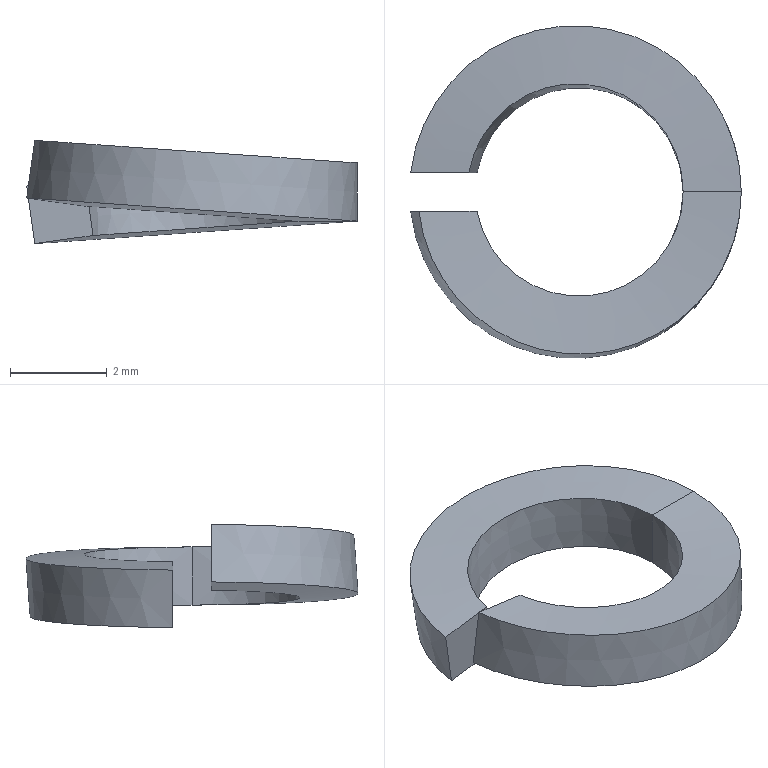Part | NX | features BREP 1 | 1 solid | 10 faces | box 6.827 x 6.867 x 2.131 mm | volume 24.116 mm3 | cone 8 | plane 2
STEP:
#1=CARTESIAN_POINT('',(-2.058,-0.4,1.498));
#2=VERTEX_POINT('',#1);
#3=CARTESIAN_POINT('',(-2.226,-0.4,0.3095));
#4=VERTEX_POINT('',#3);
#5=CARTESIAN_POINT('',(-2.058,-0.4,1.498));
#6=CARTESIAN_POINT('',(-2.084,-0.4,1.314));
#7=CARTESIAN_POINT('',(-2.11,-0.4,1.13));
#8=CARTESIAN_POINT('',(-2.161,-0.4,0.7669));
#9=CARTESIAN_POINT('',(-2.187,-0.4,0.5875));
#10=CARTESIAN_POINT('',(-2.217,-0.4,0.3753));
#11=CARTESIAN_POINT('',(-2.221,-0.4,0.3424));
#12=CARTESIAN_POINT('',(-2.226,-0.4,0.3095));
#13=B_SPLINE_CURVE_WITH_KNOTS('',3,(#5,#6,#7,#8,#9,#10,#11,#12),.UNSPECIFIED.,.F.,.F.,(4,2,2,4),(0.,0.4641,0.917,1.),.UNSPECIFIED.);
#14=EDGE_CURVE('',#2,#4,#13,.T.);
#15=ORIENTED_EDGE('',*,*,#14,.F.);
#16=CARTESIAN_POINT('',(2.2,0.,1.2));
#17=VERTEX_POINT('',#16);
#18=CARTESIAN_POINT('',(0.05246,0.,1.35));
#19=DIRECTION('',(0.06976,0.,0.9976));
#20=DIRECTION('',(0.9976,0.,-0.06976));
#21=AXIS2_PLACEMENT_3D('',#18,#19,#20);
#22=CIRCLE('',#21,2.153);
#23=EDGE_CURVE('',#2,#17,#22,.T.);
#24=ORIENTED_EDGE('',*,*,#23,.T.);
#25=CARTESIAN_POINT('',(2.2,0.,0.));
#26=VERTEX_POINT('',#25);
#27=CARTESIAN_POINT('',(2.2,0.,0.));
#28=DIRECTION('',(0.,0.,1.));
#29=VECTOR('',#28,1000.);
#30=LINE('',#27,#29);
#31=EDGE_CURVE('',#26,#17,#30,.T.);
#32=ORIENTED_EDGE('',*,*,#31,.F.);
#33=CARTESIAN_POINT('',(-0.03105,0.,0.156));
#34=DIRECTION('',(0.06976,0.,0.9976));
#35=DIRECTION('',(0.9976,0.,-0.06976));
#36=AXIS2_PLACEMENT_3D('',#33,#34,#35);
#37=CIRCLE('',#36,2.236);
#38=EDGE_CURVE('',#4,#26,#37,.T.);
#39=ORIENTED_EDGE('',*,*,#38,.F.);
#40=EDGE_LOOP('',(#15,#24,#32,#39));
#41=FACE_BOUND('',#40,.T.);
#42=CARTESIAN_POINT('',(-0.03105,0.,0.156));
#43=DIRECTION('',(-0.06976,0.,-0.9976));
#44=DIRECTION('',(0.9976,0.,-0.06976));
#45=AXIS2_PLACEMENT_3D('',#42,#43,#44);
#46=CONICAL_SURFACE('',#45,2.236,0.06981);
#47=ADVANCED_FACE('',(#41),#46,.F.);
#48=CARTESIAN_POINT('',(-3.259,-0.4,1.666));
#49=VERTEX_POINT('',#48);
#50=CARTESIAN_POINT('',(-3.259,-0.4,1.666));
#51=CARTESIAN_POINT('',(-2.859,-0.4,1.61));
#52=CARTESIAN_POINT('',(-2.458,-0.4,1.554));
#53=CARTESIAN_POINT('',(-2.058,-0.4,1.498));
#54=B_SPLINE_CURVE_WITH_KNOTS('',3,(#50,#51,#52,#53),.UNSPECIFIED.,.F.,.F.,(4,4),(0.,1.),.PIECEWISE_BEZIER_KNOTS.);
#55=EDGE_CURVE('',#49,#2,#54,.T.);
#56=ORIENTED_EDGE('',*,*,#55,.F.);
#57=CARTESIAN_POINT('',(3.4,0.,1.2));
#58=VERTEX_POINT('',#57);
#59=CARTESIAN_POINT('',(0.0583,0.,1.434));
#60=DIRECTION('',(0.06976,0.,0.9976));
#61=DIRECTION('',(0.9976,0.,-0.06976));
#62=AXIS2_PLACEMENT_3D('',#59,#60,#61);
#63=CIRCLE('',#62,3.35);
#64=EDGE_CURVE('',#49,#58,#63,.T.);
#65=ORIENTED_EDGE('',*,*,#64,.T.);
#66=CARTESIAN_POINT('',(2.2,0.,1.2));
#67=DIRECTION('',(1.,0.,0.));
#68=VECTOR('',#67,1000.);
#69=LINE('',#66,#68);
#70=EDGE_CURVE('',#17,#58,#69,.T.);
#71=ORIENTED_EDGE('',*,*,#70,.F.);
#72=ORIENTED_EDGE('',*,*,#23,.F.);
#73=EDGE_LOOP('',(#56,#65,#71,#72));
#74=FACE_BOUND('',#73,.T.);
#75=CARTESIAN_POINT('',(0.05246,0.,1.35));
#76=DIRECTION('',(0.06976,0.,0.9976));
#77=DIRECTION('',(-0.9976,0.,0.06976));
#78=AXIS2_PLACEMENT_3D('',#75,#76,#77);
#79=CONICAL_SURFACE('',#78,2.153,1.501);
#80=ADVANCED_FACE('',(#74),#79,.F.);
#81=CARTESIAN_POINT('',(-3.427,-0.4,0.4774));
#82=VERTEX_POINT('',#81);
#83=CARTESIAN_POINT('',(-3.427,-0.4,0.4774));
#84=CARTESIAN_POINT('',(-3.371,-0.4,0.8735));
#85=CARTESIAN_POINT('',(-3.315,-0.4,1.27));
#86=CARTESIAN_POINT('',(-3.259,-0.4,1.666));
#87=B_SPLINE_CURVE_WITH_KNOTS('',3,(#83,#84,#85,#86),.UNSPECIFIED.,.F.,.F.,(4,4),(0.,1.),.PIECEWISE_BEZIER_KNOTS.);
#88=EDGE_CURVE('',#82,#49,#87,.T.);
#89=ORIENTED_EDGE('',*,*,#88,.F.);
#90=CARTESIAN_POINT('',(3.4,0.,0.));
#91=VERTEX_POINT('',#90);
#92=CARTESIAN_POINT('',(-0.02521,0.,0.2395));
#93=DIRECTION('',(0.06976,0.,0.9976));
#94=DIRECTION('',(0.9976,0.,-0.06976));
#95=AXIS2_PLACEMENT_3D('',#92,#93,#94);
#96=CIRCLE('',#95,3.434);
#97=EDGE_CURVE('',#82,#91,#96,.T.);
#98=ORIENTED_EDGE('',*,*,#97,.T.);
#99=CARTESIAN_POINT('',(3.4,0.,1.2));
#100=DIRECTION('',(0.,0.,-1.));
#101=VECTOR('',#100,1000.);
#102=LINE('',#99,#101);
#103=EDGE_CURVE('',#58,#91,#102,.T.);
#104=ORIENTED_EDGE('',*,*,#103,.F.);
#105=ORIENTED_EDGE('',*,*,#64,.F.);
#106=EDGE_LOOP('',(#89,#98,#104,#105));
#107=FACE_BOUND('',#106,.T.);
#108=CARTESIAN_POINT('',(0.0583,0.,1.434));
#109=DIRECTION('',(-0.06976,0.,-0.9976));
#110=DIRECTION('',(0.9976,0.,-0.06976));
#111=AXIS2_PLACEMENT_3D('',#108,#109,#110);
#112=CONICAL_SURFACE('',#111,3.35,0.06981);
#113=ADVANCED_FACE('',(#107),#112,.T.);
#114=CARTESIAN_POINT('',(-2.226,-0.4,0.3095));
#115=CARTESIAN_POINT('',(-2.626,-0.4,0.3653));
#116=CARTESIAN_POINT('',(-3.027,-0.4,0.4213));
#117=CARTESIAN_POINT('',(-3.427,-0.4,0.4774));
#118=B_SPLINE_CURVE_WITH_KNOTS('',3,(#114,#115,#116,#117),.UNSPECIFIED.,.F.,.F.,(4,4),(0.,1.),.PIECEWISE_BEZIER_KNOTS.);
#119=EDGE_CURVE('',#4,#82,#118,.T.);
#120=ORIENTED_EDGE('',*,*,#119,.F.);
#121=ORIENTED_EDGE('',*,*,#38,.T.);
#122=CARTESIAN_POINT('',(3.4,0.,0.));
#123=DIRECTION('',(-1.,0.,0.));
#124=VECTOR('',#123,1000.);
#125=LINE('',#122,#124);
#126=EDGE_CURVE('',#91,#26,#125,.T.);
#127=ORIENTED_EDGE('',*,*,#126,.F.);
#128=ORIENTED_EDGE('',*,*,#97,.F.);
#129=EDGE_LOOP('',(#120,#121,#127,#128));
#130=FACE_BOUND('',#129,.T.);
#131=CARTESIAN_POINT('',(-0.02521,0.,0.2395));
#132=DIRECTION('',(0.06976,0.,0.9976));
#133=DIRECTION('',(-0.9976,0.,0.06976));
#134=AXIS2_PLACEMENT_3D('',#131,#132,#133);
#135=CONICAL_SURFACE('',#134,3.434,1.501);
#136=ADVANCED_FACE('',(#130),#135,.T.);
#137=CARTESIAN_POINT('',(-2.226,0.4,0.8905));
#138=VERTEX_POINT('',#137);
#139=CARTESIAN_POINT('',(-0.03105,0.,1.044));
#140=DIRECTION('',(0.06976,0.,-0.9976));
#141=DIRECTION('',(-0.9976,0.,-0.06976));
#142=AXIS2_PLACEMENT_3D('',#139,#140,#141);
#143=CIRCLE('',#142,2.236);
#144=EDGE_CURVE('',#138,#17,#143,.T.);
#145=ORIENTED_EDGE('',*,*,#144,.F.);
#146=CARTESIAN_POINT('',(-2.058,0.4,-0.2977));
#147=VERTEX_POINT('',#146);
#148=CARTESIAN_POINT('',(-2.226,0.4,0.8905));
#149=CARTESIAN_POINT('',(-2.187,0.4,0.6125));
#150=CARTESIAN_POINT('',(-2.147,0.4,0.3345));
#151=CARTESIAN_POINT('',(-2.091,0.4,-0.06158));
#152=CARTESIAN_POINT('',(-2.074,0.4,-0.1797));
#153=CARTESIAN_POINT('',(-2.058,0.4,-0.2977));
#154=B_SPLINE_CURVE_WITH_KNOTS('',3,(#148,#149,#150,#151,#152,#153),.UNSPECIFIED.,.F.,.F.,(4,2,4),(0.,0.7019,1.),.UNSPECIFIED.);
#155=EDGE_CURVE('',#138,#147,#154,.T.);
#156=ORIENTED_EDGE('',*,*,#155,.T.);
#157=CARTESIAN_POINT('',(0.05246,0.,-0.1502));
#158=DIRECTION('',(0.06976,0.,-0.9976));
#159=DIRECTION('',(-0.9976,0.,-0.06976));
#160=AXIS2_PLACEMENT_3D('',#157,#158,#159);
#161=CIRCLE('',#160,2.153);
#162=EDGE_CURVE('',#147,#26,#161,.T.);
#163=ORIENTED_EDGE('',*,*,#162,.T.);
#164=ORIENTED_EDGE('',*,*,#31,.T.);
#165=EDGE_LOOP('',(#145,#156,#163,#164));
#166=FACE_BOUND('',#165,.T.);
#167=CARTESIAN_POINT('',(0.05246,0.,-0.1502));
#168=DIRECTION('',(-0.06976,0.,0.9976));
#169=DIRECTION('',(-0.9976,0.,-0.06976));
#170=AXIS2_PLACEMENT_3D('',#167,#168,#169);
#171=CONICAL_SURFACE('',#170,2.153,0.06981);
#172=ADVANCED_FACE('',(#166),#171,.F.);
#173=CARTESIAN_POINT('',(-3.427,0.4,0.7226));
#174=VERTEX_POINT('',#173);
#175=CARTESIAN_POINT('',(-0.02521,0.,0.9605));
#176=DIRECTION('',(0.06976,0.,-0.9976));
#177=DIRECTION('',(-0.9976,0.,-0.06976));
#178=AXIS2_PLACEMENT_3D('',#175,#176,#177);
#179=CIRCLE('',#178,3.434);
#180=EDGE_CURVE('',#174,#58,#179,.T.);
#181=ORIENTED_EDGE('',*,*,#180,.F.);
#182=CARTESIAN_POINT('',(-3.427,0.4,0.7226));
#183=CARTESIAN_POINT('',(-3.027,0.4,0.7787));
#184=CARTESIAN_POINT('',(-2.626,0.4,0.8347));
#185=CARTESIAN_POINT('',(-2.226,0.4,0.8905));
#186=B_SPLINE_CURVE_WITH_KNOTS('',3,(#182,#183,#184,#185),.UNSPECIFIED.,.F.,.F.,(4,4),(0.,1.),.PIECEWISE_BEZIER_KNOTS.);
#187=EDGE_CURVE('',#174,#138,#186,.T.);
#188=ORIENTED_EDGE('',*,*,#187,.T.);
#189=ORIENTED_EDGE('',*,*,#144,.T.);
#190=ORIENTED_EDGE('',*,*,#70,.T.);
#191=EDGE_LOOP('',(#181,#188,#189,#190));
#192=FACE_BOUND('',#191,.T.);
#193=CARTESIAN_POINT('',(-0.03105,0.,1.044));
#194=DIRECTION('',(0.06976,0.,-0.9976));
#195=DIRECTION('',(0.9976,0.,0.06976));
#196=AXIS2_PLACEMENT_3D('',#193,#194,#195);
#197=CONICAL_SURFACE('',#196,2.236,1.501);
#198=ADVANCED_FACE('',(#192),#197,.T.);
#199=CARTESIAN_POINT('',(-3.259,0.4,-0.4657));
#200=VERTEX_POINT('',#199);
#201=CARTESIAN_POINT('',(0.0583,0.,-0.2337));
#202=DIRECTION('',(0.06976,0.,-0.9976));
#203=DIRECTION('',(-0.9976,0.,-0.06976));
#204=AXIS2_PLACEMENT_3D('',#201,#202,#203);
#205=CIRCLE('',#204,3.35);
#206=EDGE_CURVE('',#200,#91,#205,.T.);
#207=ORIENTED_EDGE('',*,*,#206,.F.);
#208=CARTESIAN_POINT('',(-3.259,0.4,-0.4657));
#209=CARTESIAN_POINT('',(-3.277,0.4,-0.3411));
#210=CARTESIAN_POINT('',(-3.295,0.4,-0.2165));
#211=CARTESIAN_POINT('',(-3.351,0.4,0.1796));
#212=CARTESIAN_POINT('',(-3.389,0.4,0.4511));
#213=CARTESIAN_POINT('',(-3.427,0.4,0.7226));
#214=B_SPLINE_CURVE_WITH_KNOTS('',3,(#208,#209,#210,#211,#212,#213),.UNSPECIFIED.,.F.,.F.,(4,2,4),(0.,0.3146,1.),.UNSPECIFIED.);
#215=EDGE_CURVE('',#200,#174,#214,.T.);
#216=ORIENTED_EDGE('',*,*,#215,.T.);
#217=ORIENTED_EDGE('',*,*,#180,.T.);
#218=ORIENTED_EDGE('',*,*,#103,.T.);
#219=EDGE_LOOP('',(#207,#216,#217,#218));
#220=FACE_BOUND('',#219,.T.);
#221=CARTESIAN_POINT('',(-0.02521,0.,0.9605));
#222=DIRECTION('',(-0.06976,0.,0.9976));
#223=DIRECTION('',(-0.9976,0.,-0.06976));
#224=AXIS2_PLACEMENT_3D('',#221,#222,#223);
#225=CONICAL_SURFACE('',#224,3.434,0.06981);
#226=ADVANCED_FACE('',(#220),#225,.T.);
#227=ORIENTED_EDGE('',*,*,#162,.F.);
#228=CARTESIAN_POINT('',(-2.058,0.4,-0.2977));
#229=CARTESIAN_POINT('',(-2.458,0.4,-0.3535));
#230=CARTESIAN_POINT('',(-2.859,0.4,-0.4096));
#231=CARTESIAN_POINT('',(-3.259,0.4,-0.4657));
#232=B_SPLINE_CURVE_WITH_KNOTS('',3,(#228,#229,#230,#231),.UNSPECIFIED.,.F.,.F.,(4,4),(0.,1.),.PIECEWISE_BEZIER_KNOTS.);
#233=EDGE_CURVE('',#147,#200,#232,.T.);
#234=ORIENTED_EDGE('',*,*,#233,.T.);
#235=ORIENTED_EDGE('',*,*,#206,.T.);
#236=ORIENTED_EDGE('',*,*,#126,.T.);
#237=EDGE_LOOP('',(#227,#234,#235,#236));
#238=FACE_BOUND('',#237,.T.);
#239=CARTESIAN_POINT('',(0.0583,0.,-0.2337));
#240=DIRECTION('',(0.06976,0.,-0.9976));
#241=DIRECTION('',(0.9976,0.,0.06976));
#242=AXIS2_PLACEMENT_3D('',#239,#240,#241);
#243=CONICAL_SURFACE('',#242,3.35,1.501);
#244=ADVANCED_FACE('',(#238),#243,.F.);
#245=ORIENTED_EDGE('',*,*,#187,.F.);
#246=ORIENTED_EDGE('',*,*,#215,.F.);
#247=ORIENTED_EDGE('',*,*,#233,.F.);
#248=ORIENTED_EDGE('',*,*,#155,.F.);
#249=EDGE_LOOP('',(#245,#246,#247,#248));
#250=FACE_BOUND('',#249,.T.);
#251=CARTESIAN_POINT('',(0.,0.4,-6.8));
#252=DIRECTION('',(0.,1.,0.));
#253=DIRECTION('',(0.,0.,-1.));
#254=AXIS2_PLACEMENT_3D('',#251,#252,#253);
#255=PLANE('',#254);
#256=ADVANCED_FACE('',(#250),#255,.F.);
#257=ORIENTED_EDGE('',*,*,#14,.T.);
#258=ORIENTED_EDGE('',*,*,#119,.T.);
#259=ORIENTED_EDGE('',*,*,#88,.T.);
#260=ORIENTED_EDGE('',*,*,#55,.T.);
#261=EDGE_LOOP('',(#257,#258,#259,#260));
#262=FACE_BOUND('',#261,.T.);
#263=CARTESIAN_POINT('',(-6.8,-0.4,-6.8));
#264=DIRECTION('',(0.,-1.,0.));
#265=DIRECTION('',(0.,0.,1.));
#266=AXIS2_PLACEMENT_3D('',#263,#264,#265);
#267=PLANE('',#266);
#268=ADVANCED_FACE('',(#262),#267,.F.);
#269=CLOSED_SHELL('',(#47,#80,#113,#136,#172,#198,#226,#244,#256,#268));
#270=MANIFOLD_SOLID_BREP('',#269);
#271=(LENGTH_UNIT()NAMED_UNIT(*)SI_UNIT(.MILLI.,.METRE.));
#272=UNCERTAINTY_MEASURE_WITH_UNIT(LENGTH_MEASURE(0.00001),#271,'','');
#273=(NAMED_UNIT(*)PLANE_ANGLE_UNIT()SI_UNIT($,.RADIAN.));
#274=(NAMED_UNIT(*)SI_UNIT($,.STERADIAN.)SOLID_ANGLE_UNIT());
#275=(GEOMETRIC_REPRESENTATION_CONTEXT(3)GLOBAL_UNCERTAINTY_ASSIGNED_CONTEXT((#272))GLOBAL_UNIT_ASSIGNED_CONTEXT((#271,#273,#274))REPRESENTATION_CONTEXT('',''));
#276=ADVANCED_BREP_SHAPE_REPRESENTATION('',(#270),#275);